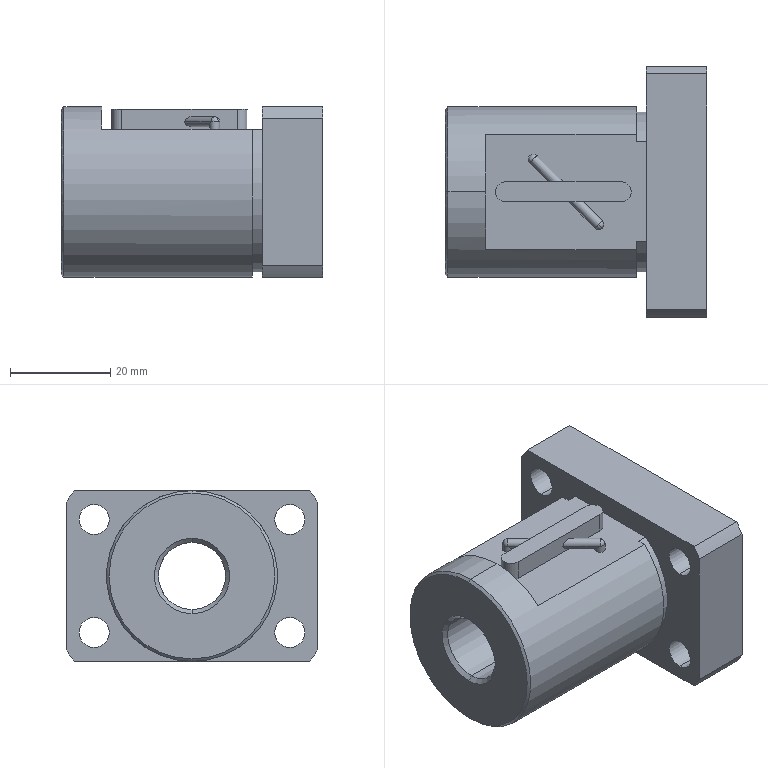Part | STEP file | Guide wheel mechanism revised.sldasm-Part-350 | 1 solid | 70 faces | box 52 x 50 x 34 mm | volume 44573 mm3 | cylinder 41 | plane 18 | cone 8 | sphere 3 | commonest cylinder face diameters 2 x8 6 x8 9.5 x8 4.917 x5 58 x4 4 x3